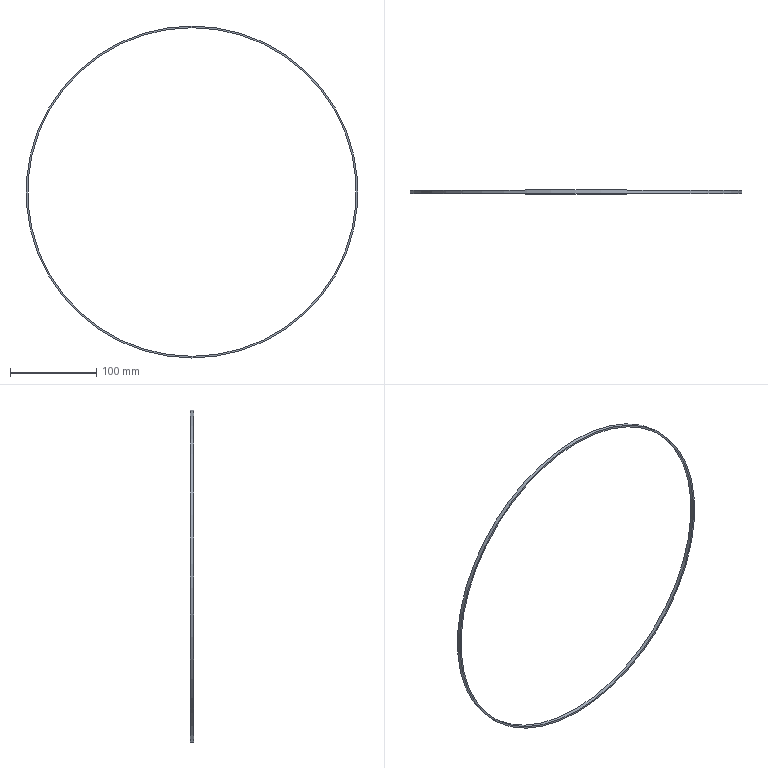Part | STEP file | Gasket | 1 solid | 4 faces | box 385 x 4 x 385 mm | volume 9626 mm3 | plane 2 | cylinder 2 | commonest cylinder face diameters 381 x1 385 x1
STEP:
#1=CARTESIAN_POINT('',(0.,2.,192.5));
#2=VERTEX_POINT('',#1);
#3=CARTESIAN_POINT('',(0.,2.,0.));
#4=DIRECTION('',(0.,1.,0.));
#5=DIRECTION('',(0.,0.,1.));
#6=AXIS2_PLACEMENT_3D('',#3,#4,#5);
#7=CIRCLE('',#6,192.5);
#8=EDGE_CURVE('',#2,#2,#7,.T.);
#9=ORIENTED_EDGE('',*,*,#8,.T.);
#10=EDGE_LOOP('',(#9));
#11=FACE_BOUND('',#10,.T.);
#12=CARTESIAN_POINT('',(0.,2.,190.5));
#13=VERTEX_POINT('',#12);
#14=CARTESIAN_POINT('',(0.,2.,0.));
#15=DIRECTION('',(0.,1.,0.));
#16=DIRECTION('',(0.,0.,1.));
#17=AXIS2_PLACEMENT_3D('',#14,#15,#16);
#18=CIRCLE('',#17,190.5);
#19=EDGE_CURVE('',#13,#13,#18,.T.);
#20=ORIENTED_EDGE('',*,*,#19,.F.);
#21=EDGE_LOOP('',(#20));
#22=FACE_BOUND('',#21,.T.);
#23=CARTESIAN_POINT('',(0.,2.,0.));
#24=DIRECTION('',(0.,1.,0.));
#25=DIRECTION('',(0.,0.,1.));
#26=AXIS2_PLACEMENT_3D('',#23,#24,#25);
#27=PLANE('',#26);
#28=ADVANCED_FACE('',(#11,#22),#27,.T.);
#29=ORIENTED_EDGE('',*,*,#8,.F.);
#30=EDGE_LOOP('',(#29));
#31=FACE_OUTER_BOUND('',#30,.T.);
#32=CARTESIAN_POINT('',(0.,-2.,192.5));
#33=VERTEX_POINT('',#32);
#34=CARTESIAN_POINT('',(0.,-2.,0.));
#35=DIRECTION('',(0.,1.,0.));
#36=DIRECTION('',(0.,0.,1.));
#37=AXIS2_PLACEMENT_3D('',#34,#35,#36);
#38=CIRCLE('',#37,192.5);
#39=EDGE_CURVE('',#33,#33,#38,.T.);
#40=ORIENTED_EDGE('',*,*,#39,.T.);
#41=EDGE_LOOP('',(#40));
#42=FACE_OUTER_BOUND('',#41,.T.);
#43=CARTESIAN_POINT('',(0.,-2.,0.));
#44=DIRECTION('',(0.,1.,0.));
#45=DIRECTION('',(0.,0.,1.));
#46=AXIS2_PLACEMENT_3D('',#43,#44,#45);
#47=CYLINDRICAL_SURFACE('',#46,192.5);
#48=ADVANCED_FACE('',(#31,#42),#47,.T.);
#49=ORIENTED_EDGE('',*,*,#39,.F.);
#50=EDGE_LOOP('',(#49));
#51=FACE_BOUND('',#50,.T.);
#52=CARTESIAN_POINT('',(0.,-2.,190.5));
#53=VERTEX_POINT('',#52);
#54=CARTESIAN_POINT('',(0.,-2.,0.));
#55=DIRECTION('',(0.,1.,0.));
#56=DIRECTION('',(0.,0.,1.));
#57=AXIS2_PLACEMENT_3D('',#54,#55,#56);
#58=CIRCLE('',#57,190.5);
#59=EDGE_CURVE('',#53,#53,#58,.T.);
#60=ORIENTED_EDGE('',*,*,#59,.T.);
#61=EDGE_LOOP('',(#60));
#62=FACE_BOUND('',#61,.T.);
#63=CARTESIAN_POINT('',(0.,-2.,0.));
#64=DIRECTION('',(0.,-1.,0.));
#65=DIRECTION('',(0.,0.,1.));
#66=AXIS2_PLACEMENT_3D('',#63,#64,#65);
#67=PLANE('',#66);
#68=ADVANCED_FACE('',(#51,#62),#67,.T.);
#69=ORIENTED_EDGE('',*,*,#19,.T.);
#70=EDGE_LOOP('',(#69));
#71=FACE_OUTER_BOUND('',#70,.T.);
#72=ORIENTED_EDGE('',*,*,#59,.F.);
#73=EDGE_LOOP('',(#72));
#74=FACE_OUTER_BOUND('',#73,.T.);
#75=CARTESIAN_POINT('',(0.,2.,0.));
#76=DIRECTION('',(0.,1.,0.));
#77=DIRECTION('',(0.,0.,1.));
#78=AXIS2_PLACEMENT_3D('',#75,#76,#77);
#79=CYLINDRICAL_SURFACE('',#78,190.5);
#80=ADVANCED_FACE('',(#71,#74),#79,.F.);
#81=CLOSED_SHELL('',(#28,#48,#68,#80));
#82=MANIFOLD_SOLID_BREP('',#81);
#83=(LENGTH_UNIT()NAMED_UNIT(*)SI_UNIT(.MILLI.,.METRE.));
#84=UNCERTAINTY_MEASURE_WITH_UNIT(LENGTH_MEASURE(0.00001),#83,'','');
#85=(NAMED_UNIT(*)PLANE_ANGLE_UNIT()SI_UNIT($,.RADIAN.));
#86=(NAMED_UNIT(*)SI_UNIT($,.STERADIAN.)SOLID_ANGLE_UNIT());
#87=(GEOMETRIC_REPRESENTATION_CONTEXT(3)GLOBAL_UNCERTAINTY_ASSIGNED_CONTEXT((#84))GLOBAL_UNIT_ASSIGNED_CONTEXT((#83,#85,#86))REPRESENTATION_CONTEXT('',''));
#88=ADVANCED_BREP_SHAPE_REPRESENTATION('',(#82),#87);